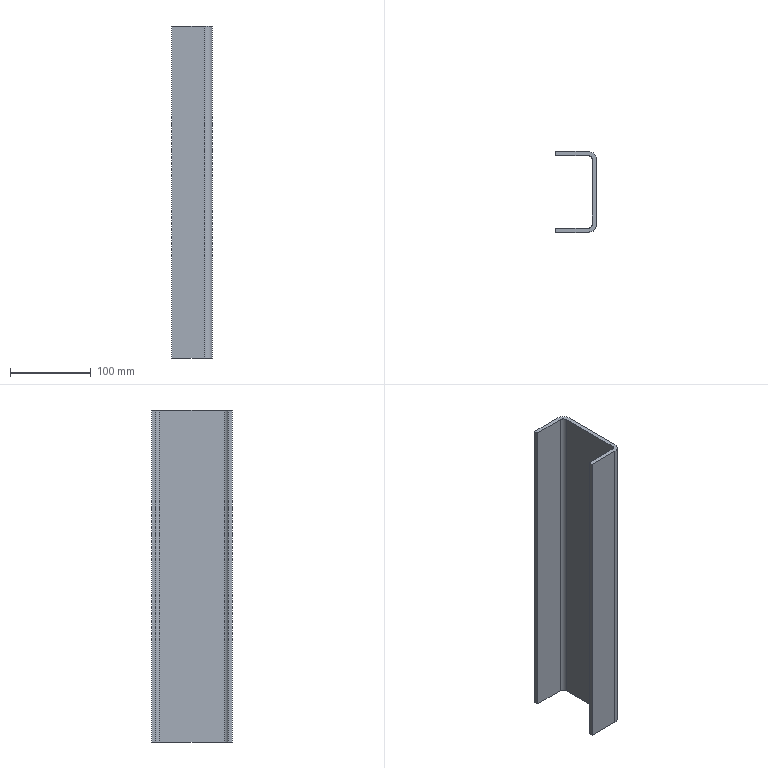Part | STEP file | 1 solid | 14 faces | box 50 x 100 x 410 mm | volume 376302 mm3 | plane 10 | cylinder 4 | commonest cylinder face diameters 10 x2 20 x2
STEP:
#1=CARTESIAN_POINT('',(0.,0.,0.));
#2=DIRECTION('',(0.,0.,1.));
#3=DIRECTION('',(1.,0.,0.));
#4=AXIS2_PLACEMENT_3D('',#1,#2,#3);
#5=CARTESIAN_POINT('',(0.,45.,-205.));
#6=VERTEX_POINT('',#5);
#7=CARTESIAN_POINT('',(0.,45.,205.));
#8=VERTEX_POINT('',#7);
#9=CARTESIAN_POINT('',(0.,45.,205.));
#10=DIRECTION('',(0.,0.,1.));
#11=VECTOR('',#10,1.);
#12=LINE('',#9,#11);
#13=CARTESIAN_POINT('',(0.,45.,205.));
#14=DIRECTION('',(1.,0.,0.));
#15=DIRECTION('',(0.,1.,0.));
#16=AXIS2_PLACEMENT_3D('',#13,#14,#15);
#17=PLANE('',#16);
#18=CARTESIAN_POINT('',(0.,0.));
#19=DIRECTION('',(0.,1.));
#20=VECTOR('',#19,1.);
#21=LINE('',#18,#20);
#22=(GEOMETRIC_REPRESENTATION_CONTEXT(2)PARAMETRIC_REPRESENTATION_CONTEXT()REPRESENTATION_CONTEXT('',''));
#23=DEFINITIONAL_REPRESENTATION('',(#21),#22);
#24=PCURVE('',#17,#23);
#25=CARTESIAN_POINT('',(40.,45.,205.));
#26=DIRECTION('',(0.,1.,0.));
#27=DIRECTION('',(1.,0.,0.));
#28=AXIS2_PLACEMENT_3D('',#25,#26,#27);
#29=PLANE('',#28);
#30=CARTESIAN_POINT('',(-40.,0.));
#31=DIRECTION('',(0.,-1.));
#32=VECTOR('',#31,1.);
#33=LINE('',#30,#32);
#34=(GEOMETRIC_REPRESENTATION_CONTEXT(2)PARAMETRIC_REPRESENTATION_CONTEXT()REPRESENTATION_CONTEXT('',''));
#35=DEFINITIONAL_REPRESENTATION('',(#33),#34);
#36=PCURVE('',#29,#35);
#37=SURFACE_CURVE('',#12,(#24,#36),.PCURVE_S1.);
#38=EDGE_CURVE('',#6,#8,#37,.T.);
#39=ORIENTED_EDGE('',*,*,#38,.T.);
#40=CARTESIAN_POINT('',(0.,50.,205.));
#41=VERTEX_POINT('',#40);
#42=CARTESIAN_POINT('',(0.,40.,205.));
#43=DIRECTION('',(0.,1.,0.));
#44=VECTOR('',#43,1.);
#45=LINE('',#42,#44);
#46=CARTESIAN_POINT('',(-5.,0.));
#47=DIRECTION('',(1.,0.));
#48=VECTOR('',#47,1.);
#49=LINE('',#46,#48);
#50=(GEOMETRIC_REPRESENTATION_CONTEXT(2)PARAMETRIC_REPRESENTATION_CONTEXT()REPRESENTATION_CONTEXT('',''));
#51=DEFINITIONAL_REPRESENTATION('',(#49),#50);
#52=PCURVE('',#17,#51);
#53=CARTESIAN_POINT('',(40.,40.,205.));
#54=DIRECTION('',(0.,0.,-1.));
#55=DIRECTION('',(0.,-1.,0.));
#56=AXIS2_PLACEMENT_3D('',#53,#54,#55);
#57=PLANE('',#56);
#58=CARTESIAN_POINT('',(0.,40.));
#59=DIRECTION('',(-1.,0.));
#60=VECTOR('',#59,1.);
#61=LINE('',#58,#60);
#62=(GEOMETRIC_REPRESENTATION_CONTEXT(2)PARAMETRIC_REPRESENTATION_CONTEXT()REPRESENTATION_CONTEXT('',''));
#63=DEFINITIONAL_REPRESENTATION('',(#61),#62);
#64=PCURVE('',#57,#63);
#65=SURFACE_CURVE('',#45,(#52,#64),.PCURVE_S1.);
#66=EDGE_CURVE('',#8,#41,#65,.T.);
#67=ORIENTED_EDGE('',*,*,#66,.T.);
#68=CARTESIAN_POINT('',(0.,50.,-205.));
#69=VERTEX_POINT('',#68);
#70=CARTESIAN_POINT('',(0.,50.,205.));
#71=DIRECTION('',(0.,0.,-1.));
#72=VECTOR('',#71,1.);
#73=LINE('',#70,#72);
#74=CARTESIAN_POINT('',(5.,0.));
#75=DIRECTION('',(0.,-1.));
#76=VECTOR('',#75,1.);
#77=LINE('',#74,#76);
#78=(GEOMETRIC_REPRESENTATION_CONTEXT(2)PARAMETRIC_REPRESENTATION_CONTEXT()REPRESENTATION_CONTEXT('',''));
#79=DEFINITIONAL_REPRESENTATION('',(#77),#78);
#80=PCURVE('',#17,#79);
#81=CARTESIAN_POINT('',(0.,50.,205.));
#82=DIRECTION('',(0.,-1.,0.));
#83=DIRECTION('',(0.,0.,-1.));
#84=AXIS2_PLACEMENT_3D('',#81,#82,#83);
#85=PLANE('',#84);
#86=CARTESIAN_POINT('',(0.,0.));
#87=DIRECTION('',(1.,0.));
#88=VECTOR('',#87,1.);
#89=LINE('',#86,#88);
#90=(GEOMETRIC_REPRESENTATION_CONTEXT(2)PARAMETRIC_REPRESENTATION_CONTEXT()REPRESENTATION_CONTEXT('',''));
#91=DEFINITIONAL_REPRESENTATION('',(#89),#90);
#92=PCURVE('',#85,#91);
#93=SURFACE_CURVE('',#73,(#80,#92),.PCURVE_S1.);
#94=EDGE_CURVE('',#41,#69,#93,.T.);
#95=ORIENTED_EDGE('',*,*,#94,.T.);
#96=CARTESIAN_POINT('',(0.,40.,-205.));
#97=DIRECTION('',(0.,1.,0.));
#98=VECTOR('',#97,1.);
#99=LINE('',#96,#98);
#100=CARTESIAN_POINT('',(-5.,-410.));
#101=DIRECTION('',(1.,0.));
#102=VECTOR('',#101,1.);
#103=LINE('',#100,#102);
#104=(GEOMETRIC_REPRESENTATION_CONTEXT(2)PARAMETRIC_REPRESENTATION_CONTEXT()REPRESENTATION_CONTEXT('',''));
#105=DEFINITIONAL_REPRESENTATION('',(#103),#104);
#106=PCURVE('',#17,#105);
#107=CARTESIAN_POINT('',(40.,40.,-205.));
#108=DIRECTION('',(0.,0.,-1.));
#109=DIRECTION('',(0.,-1.,0.));
#110=AXIS2_PLACEMENT_3D('',#107,#108,#109);
#111=PLANE('',#110);
#112=CARTESIAN_POINT('',(0.,40.));
#113=DIRECTION('',(-1.,0.));
#114=VECTOR('',#113,1.);
#115=LINE('',#112,#114);
#116=(GEOMETRIC_REPRESENTATION_CONTEXT(2)PARAMETRIC_REPRESENTATION_CONTEXT()REPRESENTATION_CONTEXT('',''));
#117=DEFINITIONAL_REPRESENTATION('',(#115),#116);
#118=PCURVE('',#111,#117);
#119=SURFACE_CURVE('',#99,(#106,#118),.PCURVE_S1.);
#120=EDGE_CURVE('',#6,#69,#119,.T.);
#121=ORIENTED_EDGE('',*,*,#120,.F.);
#122=EDGE_LOOP('',(#39,#67,#95,#121));
#123=FACE_BOUND('',#122,.T.);
#124=ADVANCED_FACE('',(#123),#17,.F.);
#125=ORIENTED_EDGE('',*,*,#94,.F.);
#126=CARTESIAN_POINT('',(40.,50.,205.));
#127=VERTEX_POINT('',#126);
#128=CARTESIAN_POINT('',(40.,50.,205.));
#129=DIRECTION('',(1.,0.,0.));
#130=VECTOR('',#129,1.);
#131=LINE('',#128,#130);
#132=CARTESIAN_POINT('',(0.,40.));
#133=DIRECTION('',(0.,1.));
#134=VECTOR('',#133,1.);
#135=LINE('',#132,#134);
#136=(GEOMETRIC_REPRESENTATION_CONTEXT(2)PARAMETRIC_REPRESENTATION_CONTEXT()REPRESENTATION_CONTEXT('',''));
#137=DEFINITIONAL_REPRESENTATION('',(#135),#136);
#138=PCURVE('',#85,#137);
#139=CARTESIAN_POINT('',(-10.,0.));
#140=DIRECTION('',(0.,-1.));
#141=VECTOR('',#140,1.);
#142=LINE('',#139,#141);
#143=(GEOMETRIC_REPRESENTATION_CONTEXT(2)PARAMETRIC_REPRESENTATION_CONTEXT()REPRESENTATION_CONTEXT('',''));
#144=DEFINITIONAL_REPRESENTATION('',(#142),#143);
#145=PCURVE('',#57,#144);
#146=SURFACE_CURVE('',#131,(#138,#145),.PCURVE_S1.);
#147=EDGE_CURVE('',#41,#127,#146,.T.);
#148=ORIENTED_EDGE('',*,*,#147,.T.);
#149=CARTESIAN_POINT('',(40.,50.,-205.));
#150=VERTEX_POINT('',#149);
#151=CARTESIAN_POINT('',(40.,50.,205.));
#152=DIRECTION('',(0.,0.,1.));
#153=VECTOR('',#152,1.);
#154=LINE('',#151,#153);
#155=CARTESIAN_POINT('',(0.,40.));
#156=DIRECTION('',(-1.,0.));
#157=VECTOR('',#156,1.);
#158=LINE('',#155,#157);
#159=(GEOMETRIC_REPRESENTATION_CONTEXT(2)PARAMETRIC_REPRESENTATION_CONTEXT()REPRESENTATION_CONTEXT('',''));
#160=DEFINITIONAL_REPRESENTATION('',(#158),#159);
#161=PCURVE('',#85,#160);
#162=CARTESIAN_POINT('',(40.,40.,205.));
#163=DIRECTION('',(0.,0.,-1.));
#164=DIRECTION('',(-1.,0.,0.));
#165=AXIS2_PLACEMENT_3D('',#162,#163,#164);
#166=CYLINDRICAL_SURFACE('',#165,10.);
#167=CARTESIAN_POINT('',(1.571,0.));
#168=DIRECTION('',(0.,-1.));
#169=VECTOR('',#168,1.);
#170=LINE('',#167,#169);
#171=(GEOMETRIC_REPRESENTATION_CONTEXT(2)PARAMETRIC_REPRESENTATION_CONTEXT()REPRESENTATION_CONTEXT('',''));
#172=DEFINITIONAL_REPRESENTATION('',(#170),#171);
#173=PCURVE('',#166,#172);
#174=SURFACE_CURVE('',#154,(#161,#173),.PCURVE_S1.);
#175=EDGE_CURVE('',#150,#127,#174,.T.);
#176=ORIENTED_EDGE('',*,*,#175,.F.);
#177=CARTESIAN_POINT('',(40.,50.,-205.));
#178=DIRECTION('',(1.,0.,0.));
#179=VECTOR('',#178,1.);
#180=LINE('',#177,#179);
#181=CARTESIAN_POINT('',(410.,40.));
#182=DIRECTION('',(0.,1.));
#183=VECTOR('',#182,1.);
#184=LINE('',#181,#183);
#185=(GEOMETRIC_REPRESENTATION_CONTEXT(2)PARAMETRIC_REPRESENTATION_CONTEXT()REPRESENTATION_CONTEXT('',''));
#186=DEFINITIONAL_REPRESENTATION('',(#184),#185);
#187=PCURVE('',#85,#186);
#188=CARTESIAN_POINT('',(-10.,0.));
#189=DIRECTION('',(0.,-1.));
#190=VECTOR('',#189,1.);
#191=LINE('',#188,#190);
#192=(GEOMETRIC_REPRESENTATION_CONTEXT(2)PARAMETRIC_REPRESENTATION_CONTEXT()REPRESENTATION_CONTEXT('',''));
#193=DEFINITIONAL_REPRESENTATION('',(#191),#192);
#194=PCURVE('',#111,#193);
#195=SURFACE_CURVE('',#180,(#187,#194),.PCURVE_S1.);
#196=EDGE_CURVE('',#69,#150,#195,.T.);
#197=ORIENTED_EDGE('',*,*,#196,.F.);
#198=EDGE_LOOP('',(#125,#148,#176,#197));
#199=FACE_BOUND('',#198,.T.);
#200=ADVANCED_FACE('',(#199),#85,.F.);
#201=CARTESIAN_POINT('',(50.,40.,205.));
#202=VERTEX_POINT('',#201);
#203=CARTESIAN_POINT('',(40.,40.,205.));
#204=DIRECTION('',(0.,0.,-1.));
#205=DIRECTION('',(-1.,0.,0.));
#206=AXIS2_PLACEMENT_3D('',#203,#204,#205);
#207=CIRCLE('',#206,10.);
#208=CARTESIAN_POINT('',(0.,0.));
#209=DIRECTION('',(1.,0.));
#210=VECTOR('',#209,1.);
#211=LINE('',#208,#210);
#212=(GEOMETRIC_REPRESENTATION_CONTEXT(2)PARAMETRIC_REPRESENTATION_CONTEXT()REPRESENTATION_CONTEXT('',''));
#213=DEFINITIONAL_REPRESENTATION('',(#211),#212);
#214=PCURVE('',#166,#213);
#215=CARTESIAN_POINT('',(0.,0.));
#216=DIRECTION('',(0.,1.));
#217=AXIS2_PLACEMENT_2D('',#215,#216);
#218=CIRCLE('',#217,10.);
#219=(GEOMETRIC_REPRESENTATION_CONTEXT(2)PARAMETRIC_REPRESENTATION_CONTEXT()REPRESENTATION_CONTEXT('',''));
#220=DEFINITIONAL_REPRESENTATION('',(#218),#219);
#221=PCURVE('',#57,#220);
#222=SURFACE_CURVE('',#207,(#214,#221),.PCURVE_S1.);
#223=EDGE_CURVE('',#127,#202,#222,.T.);
#224=ORIENTED_EDGE('',*,*,#223,.T.);
#225=CARTESIAN_POINT('',(50.,40.,-205.));
#226=VERTEX_POINT('',#225);
#227=CARTESIAN_POINT('',(50.,40.,205.));
#228=DIRECTION('',(0.,0.,-1.));
#229=VECTOR('',#228,1.);
#230=LINE('',#227,#229);
#231=CARTESIAN_POINT('',(3.142,0.));
#232=DIRECTION('',(0.,1.));
#233=VECTOR('',#232,1.);
#234=LINE('',#231,#233);
#235=(GEOMETRIC_REPRESENTATION_CONTEXT(2)PARAMETRIC_REPRESENTATION_CONTEXT()REPRESENTATION_CONTEXT('',''));
#236=DEFINITIONAL_REPRESENTATION('',(#234),#235);
#237=PCURVE('',#166,#236);
#238=CARTESIAN_POINT('',(50.,40.,205.));
#239=DIRECTION('',(-1.,0.,0.));
#240=DIRECTION('',(0.,1.,0.));
#241=AXIS2_PLACEMENT_3D('',#238,#239,#240);
#242=PLANE('',#241);
#243=CARTESIAN_POINT('',(0.,0.));
#244=DIRECTION('',(0.,1.));
#245=VECTOR('',#244,1.);
#246=LINE('',#243,#245);
#247=(GEOMETRIC_REPRESENTATION_CONTEXT(2)PARAMETRIC_REPRESENTATION_CONTEXT()REPRESENTATION_CONTEXT('',''));
#248=DEFINITIONAL_REPRESENTATION('',(#246),#247);
#249=PCURVE('',#242,#248);
#250=SURFACE_CURVE('',#230,(#237,#249),.PCURVE_S1.);
#251=EDGE_CURVE('',#202,#226,#250,.T.);
#252=ORIENTED_EDGE('',*,*,#251,.T.);
#253=CARTESIAN_POINT('',(40.,40.,-205.));
#254=DIRECTION('',(0.,0.,-1.));
#255=DIRECTION('',(-1.,0.,0.));
#256=AXIS2_PLACEMENT_3D('',#253,#254,#255);
#257=CIRCLE('',#256,10.);
#258=CARTESIAN_POINT('',(0.,410.));
#259=DIRECTION('',(1.,0.));
#260=VECTOR('',#259,1.);
#261=LINE('',#258,#260);
#262=(GEOMETRIC_REPRESENTATION_CONTEXT(2)PARAMETRIC_REPRESENTATION_CONTEXT()REPRESENTATION_CONTEXT('',''));
#263=DEFINITIONAL_REPRESENTATION('',(#261),#262);
#264=PCURVE('',#166,#263);
#265=CARTESIAN_POINT('',(0.,0.));
#266=DIRECTION('',(0.,1.));
#267=AXIS2_PLACEMENT_2D('',#265,#266);
#268=CIRCLE('',#267,10.);
#269=(GEOMETRIC_REPRESENTATION_CONTEXT(2)PARAMETRIC_REPRESENTATION_CONTEXT()REPRESENTATION_CONTEXT('',''));
#270=DEFINITIONAL_REPRESENTATION('',(#268),#269);
#271=PCURVE('',#111,#270);
#272=SURFACE_CURVE('',#257,(#264,#271),.PCURVE_S1.);
#273=EDGE_CURVE('',#150,#226,#272,.T.);
#274=ORIENTED_EDGE('',*,*,#273,.F.);
#275=ORIENTED_EDGE('',*,*,#175,.T.);
#276=EDGE_LOOP('',(#224,#252,#274,#275));
#277=FACE_BOUND('',#276,.T.);
#278=ADVANCED_FACE('',(#277),#166,.T.);
#279=ORIENTED_EDGE('',*,*,#251,.F.);
#280=CARTESIAN_POINT('',(50.,-40.,205.));
#281=VERTEX_POINT('',#280);
#282=CARTESIAN_POINT('',(50.,40.,205.));
#283=DIRECTION('',(0.,-1.,0.));
#284=VECTOR('',#283,1.);
#285=LINE('',#282,#284);
#286=CARTESIAN_POINT('',(0.,0.));
#287=DIRECTION('',(-1.,0.));
#288=VECTOR('',#287,1.);
#289=LINE('',#286,#288);
#290=(GEOMETRIC_REPRESENTATION_CONTEXT(2)PARAMETRIC_REPRESENTATION_CONTEXT()REPRESENTATION_CONTEXT('',''));
#291=DEFINITIONAL_REPRESENTATION('',(#289),#290);
#292=PCURVE('',#242,#291);
#293=CARTESIAN_POINT('',(0.,-10.));
#294=DIRECTION('',(1.,0.));
#295=VECTOR('',#294,1.);
#296=LINE('',#293,#295);
#297=(GEOMETRIC_REPRESENTATION_CONTEXT(2)PARAMETRIC_REPRESENTATION_CONTEXT()REPRESENTATION_CONTEXT('',''));
#298=DEFINITIONAL_REPRESENTATION('',(#296),#297);
#299=PCURVE('',#57,#298);
#300=SURFACE_CURVE('',#285,(#292,#299),.PCURVE_S1.);
#301=EDGE_CURVE('',#202,#281,#300,.T.);
#302=ORIENTED_EDGE('',*,*,#301,.T.);
#303=CARTESIAN_POINT('',(50.,-40.,-205.));
#304=VERTEX_POINT('',#303);
#305=CARTESIAN_POINT('',(50.,-40.,205.));
#306=DIRECTION('',(0.,0.,1.));
#307=VECTOR('',#306,1.);
#308=LINE('',#305,#307);
#309=CARTESIAN_POINT('',(-80.,0.));
#310=DIRECTION('',(0.,-1.));
#311=VECTOR('',#310,1.);
#312=LINE('',#309,#311);
#313=(GEOMETRIC_REPRESENTATION_CONTEXT(2)PARAMETRIC_REPRESENTATION_CONTEXT()REPRESENTATION_CONTEXT('',''));
#314=DEFINITIONAL_REPRESENTATION('',(#312),#313);
#315=PCURVE('',#242,#314);
#316=CARTESIAN_POINT('',(40.,-40.,205.));
#317=DIRECTION('',(0.,0.,-1.));
#318=DIRECTION('',(-1.,0.,0.));
#319=AXIS2_PLACEMENT_3D('',#316,#317,#318);
#320=CYLINDRICAL_SURFACE('',#319,10.);
#321=CARTESIAN_POINT('',(3.142,0.));
#322=DIRECTION('',(0.,-1.));
#323=VECTOR('',#322,1.);
#324=LINE('',#321,#323);
#325=(GEOMETRIC_REPRESENTATION_CONTEXT(2)PARAMETRIC_REPRESENTATION_CONTEXT()REPRESENTATION_CONTEXT('',''));
#326=DEFINITIONAL_REPRESENTATION('',(#324),#325);
#327=PCURVE('',#320,#326);
#328=SURFACE_CURVE('',#308,(#315,#327),.PCURVE_S1.);
#329=EDGE_CURVE('',#304,#281,#328,.T.);
#330=ORIENTED_EDGE('',*,*,#329,.F.);
#331=CARTESIAN_POINT('',(50.,40.,-205.));
#332=DIRECTION('',(0.,-1.,0.));
#333=VECTOR('',#332,1.);
#334=LINE('',#331,#333);
#335=CARTESIAN_POINT('',(0.,410.));
#336=DIRECTION('',(-1.,0.));
#337=VECTOR('',#336,1.);
#338=LINE('',#335,#337);
#339=(GEOMETRIC_REPRESENTATION_CONTEXT(2)PARAMETRIC_REPRESENTATION_CONTEXT()REPRESENTATION_CONTEXT('',''));
#340=DEFINITIONAL_REPRESENTATION('',(#338),#339);
#341=PCURVE('',#242,#340);
#342=CARTESIAN_POINT('',(0.,-10.));
#343=DIRECTION('',(1.,0.));
#344=VECTOR('',#343,1.);
#345=LINE('',#342,#344);
#346=(GEOMETRIC_REPRESENTATION_CONTEXT(2)PARAMETRIC_REPRESENTATION_CONTEXT()REPRESENTATION_CONTEXT('',''));
#347=DEFINITIONAL_REPRESENTATION('',(#345),#346);
#348=PCURVE('',#111,#347);
#349=SURFACE_CURVE('',#334,(#341,#348),.PCURVE_S1.);
#350=EDGE_CURVE('',#226,#304,#349,.T.);
#351=ORIENTED_EDGE('',*,*,#350,.F.);
#352=EDGE_LOOP('',(#279,#302,#330,#351));
#353=FACE_BOUND('',#352,.T.);
#354=ADVANCED_FACE('',(#353),#242,.F.);
#355=CARTESIAN_POINT('',(40.,-50.,205.));
#356=VERTEX_POINT('',#355);
#357=CARTESIAN_POINT('',(40.,-40.,205.));
#358=DIRECTION('',(0.,0.,-1.));
#359=DIRECTION('',(-1.,0.,0.));
#360=AXIS2_PLACEMENT_3D('',#357,#358,#359);
#361=CIRCLE('',#360,10.);
#362=CARTESIAN_POINT('',(0.,0.));
#363=DIRECTION('',(1.,0.));
#364=VECTOR('',#363,1.);
#365=LINE('',#362,#364);
#366=(GEOMETRIC_REPRESENTATION_CONTEXT(2)PARAMETRIC_REPRESENTATION_CONTEXT()REPRESENTATION_CONTEXT('',''));
#367=DEFINITIONAL_REPRESENTATION('',(#365),#366);
#368=PCURVE('',#320,#367);
#369=CARTESIAN_POINT('',(80.,0.));
#370=DIRECTION('',(0.,1.));
#371=AXIS2_PLACEMENT_2D('',#369,#370);
#372=CIRCLE('',#371,10.);
#373=(GEOMETRIC_REPRESENTATION_CONTEXT(2)PARAMETRIC_REPRESENTATION_CONTEXT()REPRESENTATION_CONTEXT('',''));
#374=DEFINITIONAL_REPRESENTATION('',(#372),#373);
#375=PCURVE('',#57,#374);
#376=SURFACE_CURVE('',#361,(#368,#375),.PCURVE_S1.);
#377=EDGE_CURVE('',#281,#356,#376,.T.);
#378=ORIENTED_EDGE('',*,*,#377,.T.);
#379=CARTESIAN_POINT('',(40.,-50.,-205.));
#380=VERTEX_POINT('',#379);
#381=CARTESIAN_POINT('',(40.,-50.,205.));
#382=DIRECTION('',(0.,0.,-1.));
#383=VECTOR('',#382,1.);
#384=LINE('',#381,#383);
#385=CARTESIAN_POINT('',(4.712,0.));
#386=DIRECTION('',(0.,1.));
#387=VECTOR('',#386,1.);
#388=LINE('',#385,#387);
#389=(GEOMETRIC_REPRESENTATION_CONTEXT(2)PARAMETRIC_REPRESENTATION_CONTEXT()REPRESENTATION_CONTEXT('',''));
#390=DEFINITIONAL_REPRESENTATION('',(#388),#389);
#391=PCURVE('',#320,#390);
#392=CARTESIAN_POINT('',(40.,-50.,205.));
#393=DIRECTION('',(0.,1.,0.));
#394=DIRECTION('',(1.,0.,0.));
#395=AXIS2_PLACEMENT_3D('',#392,#393,#394);
#396=PLANE('',#395);
#397=CARTESIAN_POINT('',(0.,0.));
#398=DIRECTION('',(0.,1.));
#399=VECTOR('',#398,1.);
#400=LINE('',#397,#399);
#401=(GEOMETRIC_REPRESENTATION_CONTEXT(2)PARAMETRIC_REPRESENTATION_CONTEXT()REPRESENTATION_CONTEXT('',''));
#402=DEFINITIONAL_REPRESENTATION('',(#400),#401);
#403=PCURVE('',#396,#402);
#404=SURFACE_CURVE('',#384,(#391,#403),.PCURVE_S1.);
#405=EDGE_CURVE('',#356,#380,#404,.T.);
#406=ORIENTED_EDGE('',*,*,#405,.T.);
#407=CARTESIAN_POINT('',(40.,-40.,-205.));
#408=DIRECTION('',(0.,0.,-1.));
#409=DIRECTION('',(-1.,0.,0.));
#410=AXIS2_PLACEMENT_3D('',#407,#408,#409);
#411=CIRCLE('',#410,10.);
#412=CARTESIAN_POINT('',(0.,410.));
#413=DIRECTION('',(1.,0.));
#414=VECTOR('',#413,1.);
#415=LINE('',#412,#414);
#416=(GEOMETRIC_REPRESENTATION_CONTEXT(2)PARAMETRIC_REPRESENTATION_CONTEXT()REPRESENTATION_CONTEXT('',''));
#417=DEFINITIONAL_REPRESENTATION('',(#415),#416);
#418=PCURVE('',#320,#417);
#419=CARTESIAN_POINT('',(80.,0.));
#420=DIRECTION('',(0.,1.));
#421=AXIS2_PLACEMENT_2D('',#419,#420);
#422=CIRCLE('',#421,10.);
#423=(GEOMETRIC_REPRESENTATION_CONTEXT(2)PARAMETRIC_REPRESENTATION_CONTEXT()REPRESENTATION_CONTEXT('',''));
#424=DEFINITIONAL_REPRESENTATION('',(#422),#423);
#425=PCURVE('',#111,#424);
#426=SURFACE_CURVE('',#411,(#418,#425),.PCURVE_S1.);
#427=EDGE_CURVE('',#304,#380,#426,.T.);
#428=ORIENTED_EDGE('',*,*,#427,.F.);
#429=ORIENTED_EDGE('',*,*,#329,.T.);
#430=EDGE_LOOP('',(#378,#406,#428,#429));
#431=FACE_BOUND('',#430,.T.);
#432=ADVANCED_FACE('',(#431),#320,.T.);
#433=ORIENTED_EDGE('',*,*,#405,.F.);
#434=CARTESIAN_POINT('',(0.,-50.,205.));
#435=VERTEX_POINT('',#434);
#436=CARTESIAN_POINT('',(40.,-50.,205.));
#437=DIRECTION('',(-1.,0.,0.));
#438=VECTOR('',#437,1.);
#439=LINE('',#436,#438);
#440=CARTESIAN_POINT('',(0.,0.));
#441=DIRECTION('',(-1.,0.));
#442=VECTOR('',#441,1.);
#443=LINE('',#440,#442);
#444=(GEOMETRIC_REPRESENTATION_CONTEXT(2)PARAMETRIC_REPRESENTATION_CONTEXT()REPRESENTATION_CONTEXT('',''));
#445=DEFINITIONAL_REPRESENTATION('',(#443),#444);
#446=PCURVE('',#396,#445);
#447=CARTESIAN_POINT('',(90.,0.));
#448=DIRECTION('',(0.,1.));
#449=VECTOR('',#448,1.);
#450=LINE('',#447,#449);
#451=(GEOMETRIC_REPRESENTATION_CONTEXT(2)PARAMETRIC_REPRESENTATION_CONTEXT()REPRESENTATION_CONTEXT('',''));
#452=DEFINITIONAL_REPRESENTATION('',(#450),#451);
#453=PCURVE('',#57,#452);
#454=SURFACE_CURVE('',#439,(#446,#453),.PCURVE_S1.);
#455=EDGE_CURVE('',#356,#435,#454,.T.);
#456=ORIENTED_EDGE('',*,*,#455,.T.);
#457=CARTESIAN_POINT('',(0.,-50.,-205.));
#458=VERTEX_POINT('',#457);
#459=CARTESIAN_POINT('',(0.,-50.,205.));
#460=DIRECTION('',(0.,0.,-1.));
#461=VECTOR('',#460,1.);
#462=LINE('',#459,#461);
#463=CARTESIAN_POINT('',(-40.,0.));
#464=DIRECTION('',(0.,1.));
#465=VECTOR('',#464,1.);
#466=LINE('',#463,#465);
#467=(GEOMETRIC_REPRESENTATION_CONTEXT(2)PARAMETRIC_REPRESENTATION_CONTEXT()REPRESENTATION_CONTEXT('',''));
#468=DEFINITIONAL_REPRESENTATION('',(#466),#467);
#469=PCURVE('',#396,#468);
#470=CARTESIAN_POINT('',(0.,-50.,205.));
#471=DIRECTION('',(1.,0.,0.));
#472=DIRECTION('',(0.,1.,0.));
#473=AXIS2_PLACEMENT_3D('',#470,#471,#472);
#474=PLANE('',#473);
#475=CARTESIAN_POINT('',(0.,0.));
#476=DIRECTION('',(0.,-1.));
#477=VECTOR('',#476,1.);
#478=LINE('',#475,#477);
#479=(GEOMETRIC_REPRESENTATION_CONTEXT(2)PARAMETRIC_REPRESENTATION_CONTEXT()REPRESENTATION_CONTEXT('',''));
#480=DEFINITIONAL_REPRESENTATION('',(#478),#479);
#481=PCURVE('',#474,#480);
#482=SURFACE_CURVE('',#462,(#469,#481),.PCURVE_S1.);
#483=EDGE_CURVE('',#435,#458,#482,.T.);
#484=ORIENTED_EDGE('',*,*,#483,.T.);
#485=CARTESIAN_POINT('',(40.,-50.,-205.));
#486=DIRECTION('',(-1.,0.,0.));
#487=VECTOR('',#486,1.);
#488=LINE('',#485,#487);
#489=CARTESIAN_POINT('',(0.,410.));
#490=DIRECTION('',(-1.,0.));
#491=VECTOR('',#490,1.);
#492=LINE('',#489,#491);
#493=(GEOMETRIC_REPRESENTATION_CONTEXT(2)PARAMETRIC_REPRESENTATION_CONTEXT()REPRESENTATION_CONTEXT('',''));
#494=DEFINITIONAL_REPRESENTATION('',(#492),#493);
#495=PCURVE('',#396,#494);
#496=CARTESIAN_POINT('',(90.,0.));
#497=DIRECTION('',(0.,1.));
#498=VECTOR('',#497,1.);
#499=LINE('',#496,#498);
#500=(GEOMETRIC_REPRESENTATION_CONTEXT(2)PARAMETRIC_REPRESENTATION_CONTEXT()REPRESENTATION_CONTEXT('',''));
#501=DEFINITIONAL_REPRESENTATION('',(#499),#500);
#502=PCURVE('',#111,#501);
#503=SURFACE_CURVE('',#488,(#495,#502),.PCURVE_S1.);
#504=EDGE_CURVE('',#380,#458,#503,.T.);
#505=ORIENTED_EDGE('',*,*,#504,.F.);
#506=EDGE_LOOP('',(#433,#456,#484,#505));
#507=FACE_BOUND('',#506,.T.);
#508=ADVANCED_FACE('',(#507),#396,.F.);
#509=ORIENTED_EDGE('',*,*,#483,.F.);
#510=CARTESIAN_POINT('',(0.,-45.,205.));
#511=VERTEX_POINT('',#510);
#512=CARTESIAN_POINT('',(0.,40.,205.));
#513=DIRECTION('',(0.,1.,0.));
#514=VECTOR('',#513,1.);
#515=LINE('',#512,#514);
#516=CARTESIAN_POINT('',(90.,0.));
#517=DIRECTION('',(1.,0.));
#518=VECTOR('',#517,1.);
#519=LINE('',#516,#518);
#520=(GEOMETRIC_REPRESENTATION_CONTEXT(2)PARAMETRIC_REPRESENTATION_CONTEXT()REPRESENTATION_CONTEXT('',''));
#521=DEFINITIONAL_REPRESENTATION('',(#519),#520);
#522=PCURVE('',#474,#521);
#523=CARTESIAN_POINT('',(0.,40.));
#524=DIRECTION('',(-1.,0.));
#525=VECTOR('',#524,1.);
#526=LINE('',#523,#525);
#527=(GEOMETRIC_REPRESENTATION_CONTEXT(2)PARAMETRIC_REPRESENTATION_CONTEXT()REPRESENTATION_CONTEXT('',''));
#528=DEFINITIONAL_REPRESENTATION('',(#526),#527);
#529=PCURVE('',#57,#528);
#530=SURFACE_CURVE('',#515,(#522,#529),.PCURVE_S1.);
#531=EDGE_CURVE('',#435,#511,#530,.T.);
#532=ORIENTED_EDGE('',*,*,#531,.T.);
#533=CARTESIAN_POINT('',(0.,-45.,-205.));
#534=VERTEX_POINT('',#533);
#535=CARTESIAN_POINT('',(0.,-45.,205.));
#536=DIRECTION('',(0.,0.,-1.));
#537=VECTOR('',#536,1.);
#538=LINE('',#535,#537);
#539=CARTESIAN_POINT('',(5.,0.));
#540=DIRECTION('',(0.,-1.));
#541=VECTOR('',#540,1.);
#542=LINE('',#539,#541);
#543=(GEOMETRIC_REPRESENTATION_CONTEXT(2)PARAMETRIC_REPRESENTATION_CONTEXT()REPRESENTATION_CONTEXT('',''));
#544=DEFINITIONAL_REPRESENTATION('',(#542),#543);
#545=PCURVE('',#474,#544);
#546=CARTESIAN_POINT('',(0.,-45.,205.));
#547=DIRECTION('',(0.,-1.,0.));
#548=DIRECTION('',(0.,0.,-1.));
#549=AXIS2_PLACEMENT_3D('',#546,#547,#548);
#550=PLANE('',#549);
#551=CARTESIAN_POINT('',(0.,0.));
#552=DIRECTION('',(1.,0.));
#553=VECTOR('',#552,1.);
#554=LINE('',#551,#553);
#555=(GEOMETRIC_REPRESENTATION_CONTEXT(2)PARAMETRIC_REPRESENTATION_CONTEXT()REPRESENTATION_CONTEXT('',''));
#556=DEFINITIONAL_REPRESENTATION('',(#554),#555);
#557=PCURVE('',#550,#556);
#558=SURFACE_CURVE('',#538,(#545,#557),.PCURVE_S1.);
#559=EDGE_CURVE('',#511,#534,#558,.T.);
#560=ORIENTED_EDGE('',*,*,#559,.T.);
#561=CARTESIAN_POINT('',(0.,40.,-205.));
#562=DIRECTION('',(0.,1.,0.));
#563=VECTOR('',#562,1.);
#564=LINE('',#561,#563);
#565=CARTESIAN_POINT('',(90.,-410.));
#566=DIRECTION('',(1.,0.));
#567=VECTOR('',#566,1.);
#568=LINE('',#565,#567);
#569=(GEOMETRIC_REPRESENTATION_CONTEXT(2)PARAMETRIC_REPRESENTATION_CONTEXT()REPRESENTATION_CONTEXT('',''));
#570=DEFINITIONAL_REPRESENTATION('',(#568),#569);
#571=PCURVE('',#474,#570);
#572=CARTESIAN_POINT('',(0.,40.));
#573=DIRECTION('',(-1.,0.));
#574=VECTOR('',#573,1.);
#575=LINE('',#572,#574);
#576=(GEOMETRIC_REPRESENTATION_CONTEXT(2)PARAMETRIC_REPRESENTATION_CONTEXT()REPRESENTATION_CONTEXT('',''));
#577=DEFINITIONAL_REPRESENTATION('',(#575),#576);
#578=PCURVE('',#111,#577);
#579=SURFACE_CURVE('',#564,(#571,#578),.PCURVE_S1.);
#580=EDGE_CURVE('',#458,#534,#579,.T.);
#581=ORIENTED_EDGE('',*,*,#580,.F.);
#582=EDGE_LOOP('',(#509,#532,#560,#581));
#583=FACE_BOUND('',#582,.T.);
#584=ADVANCED_FACE('',(#583),#474,.F.);
#585=ORIENTED_EDGE('',*,*,#559,.F.);
#586=CARTESIAN_POINT('',(40.,-45.,205.));
#587=VERTEX_POINT('',#586);
#588=CARTESIAN_POINT('',(40.,-45.,205.));
#589=DIRECTION('',(1.,0.,0.));
#590=VECTOR('',#589,1.);
#591=LINE('',#588,#590);
#592=CARTESIAN_POINT('',(0.,40.));
#593=DIRECTION('',(0.,1.));
#594=VECTOR('',#593,1.);
#595=LINE('',#592,#594);
#596=(GEOMETRIC_REPRESENTATION_CONTEXT(2)PARAMETRIC_REPRESENTATION_CONTEXT()REPRESENTATION_CONTEXT('',''));
#597=DEFINITIONAL_REPRESENTATION('',(#595),#596);
#598=PCURVE('',#550,#597);
#599=CARTESIAN_POINT('',(85.,0.));
#600=DIRECTION('',(0.,-1.));
#601=VECTOR('',#600,1.);
#602=LINE('',#599,#601);
#603=(GEOMETRIC_REPRESENTATION_CONTEXT(2)PARAMETRIC_REPRESENTATION_CONTEXT()REPRESENTATION_CONTEXT('',''));
#604=DEFINITIONAL_REPRESENTATION('',(#602),#603);
#605=PCURVE('',#57,#604);
#606=SURFACE_CURVE('',#591,(#598,#605),.PCURVE_S1.);
#607=EDGE_CURVE('',#511,#587,#606,.T.);
#608=ORIENTED_EDGE('',*,*,#607,.T.);
#609=CARTESIAN_POINT('',(40.,-45.,-205.));
#610=VERTEX_POINT('',#609);
#611=CARTESIAN_POINT('',(40.,-45.,205.));
#612=DIRECTION('',(0.,0.,-1.));
#613=VECTOR('',#612,1.);
#614=LINE('',#611,#613);
#615=CARTESIAN_POINT('',(0.,40.));
#616=DIRECTION('',(1.,0.));
#617=VECTOR('',#616,1.);
#618=LINE('',#615,#617);
#619=(GEOMETRIC_REPRESENTATION_CONTEXT(2)PARAMETRIC_REPRESENTATION_CONTEXT()REPRESENTATION_CONTEXT('',''));
#620=DEFINITIONAL_REPRESENTATION('',(#618),#619);
#621=PCURVE('',#550,#620);
#622=CARTESIAN_POINT('',(40.,-40.,205.));
#623=DIRECTION('',(0.,0.,-1.));
#624=DIRECTION('',(-1.,0.,0.));
#625=AXIS2_PLACEMENT_3D('',#622,#623,#624);
#626=CYLINDRICAL_SURFACE('',#625,5.);
#627=CARTESIAN_POINT('',(4.712,0.));
#628=DIRECTION('',(0.,1.));
#629=VECTOR('',#628,1.);
#630=LINE('',#627,#629);
#631=(GEOMETRIC_REPRESENTATION_CONTEXT(2)PARAMETRIC_REPRESENTATION_CONTEXT()REPRESENTATION_CONTEXT('',''));
#632=DEFINITIONAL_REPRESENTATION('',(#630),#631);
#633=PCURVE('',#626,#632);
#634=SURFACE_CURVE('',#614,(#621,#633),.PCURVE_S1.);
#635=EDGE_CURVE('',#587,#610,#634,.T.);
#636=ORIENTED_EDGE('',*,*,#635,.T.);
#637=CARTESIAN_POINT('',(40.,-45.,-205.));
#638=DIRECTION('',(1.,0.,0.));
#639=VECTOR('',#638,1.);
#640=LINE('',#637,#639);
#641=CARTESIAN_POINT('',(410.,40.));
#642=DIRECTION('',(0.,1.));
#643=VECTOR('',#642,1.);
#644=LINE('',#641,#643);
#645=(GEOMETRIC_REPRESENTATION_CONTEXT(2)PARAMETRIC_REPRESENTATION_CONTEXT()REPRESENTATION_CONTEXT('',''));
#646=DEFINITIONAL_REPRESENTATION('',(#644),#645);
#647=PCURVE('',#550,#646);
#648=CARTESIAN_POINT('',(85.,0.));
#649=DIRECTION('',(0.,-1.));
#650=VECTOR('',#649,1.);
#651=LINE('',#648,#650);
#652=(GEOMETRIC_REPRESENTATION_CONTEXT(2)PARAMETRIC_REPRESENTATION_CONTEXT()REPRESENTATION_CONTEXT('',''));
#653=DEFINITIONAL_REPRESENTATION('',(#651),#652);
#654=PCURVE('',#111,#653);
#655=SURFACE_CURVE('',#640,(#647,#654),.PCURVE_S1.);
#656=EDGE_CURVE('',#534,#610,#655,.T.);
#657=ORIENTED_EDGE('',*,*,#656,.F.);
#658=EDGE_LOOP('',(#585,#608,#636,#657));
#659=FACE_BOUND('',#658,.T.);
#660=ADVANCED_FACE('',(#659),#550,.F.);
#661=CARTESIAN_POINT('',(40.,45.,-205.));
#662=VERTEX_POINT('',#661);
#663=CARTESIAN_POINT('',(40.,45.,205.));
#664=VERTEX_POINT('',#663);
#665=CARTESIAN_POINT('',(40.,45.,205.));
#666=DIRECTION('',(0.,0.,1.));
#667=VECTOR('',#666,1.);
#668=LINE('',#665,#667);
#669=CARTESIAN_POINT('',(0.,0.));
#670=DIRECTION('',(0.,-1.));
#671=VECTOR('',#670,1.);
#672=LINE('',#669,#671);
#673=(GEOMETRIC_REPRESENTATION_CONTEXT(2)PARAMETRIC_REPRESENTATION_CONTEXT()REPRESENTATION_CONTEXT('',''));
#674=DEFINITIONAL_REPRESENTATION('',(#672),#673);
#675=PCURVE('',#29,#674);
#676=CARTESIAN_POINT('',(40.,40.,205.));
#677=DIRECTION('',(0.,0.,-1.));
#678=DIRECTION('',(-1.,0.,0.));
#679=AXIS2_PLACEMENT_3D('',#676,#677,#678);
#680=CYLINDRICAL_SURFACE('',#679,5.);
#681=CARTESIAN_POINT('',(1.571,0.));
#682=DIRECTION('',(0.,-1.));
#683=VECTOR('',#682,1.);
#684=LINE('',#681,#683);
#685=(GEOMETRIC_REPRESENTATION_CONTEXT(2)PARAMETRIC_REPRESENTATION_CONTEXT()REPRESENTATION_CONTEXT('',''));
#686=DEFINITIONAL_REPRESENTATION('',(#684),#685);
#687=PCURVE('',#680,#686);
#688=SURFACE_CURVE('',#668,(#675,#687),.PCURVE_S1.);
#689=EDGE_CURVE('',#662,#664,#688,.T.);
#690=ORIENTED_EDGE('',*,*,#689,.T.);
#691=CARTESIAN_POINT('',(40.,45.,205.));
#692=DIRECTION('',(-1.,0.,0.));
#693=VECTOR('',#692,1.);
#694=LINE('',#691,#693);
#695=CARTESIAN_POINT('',(0.,0.));
#696=DIRECTION('',(-1.,0.));
#697=VECTOR('',#696,1.);
#698=LINE('',#695,#697);
#699=(GEOMETRIC_REPRESENTATION_CONTEXT(2)PARAMETRIC_REPRESENTATION_CONTEXT()REPRESENTATION_CONTEXT('',''));
#700=DEFINITIONAL_REPRESENTATION('',(#698),#699);
#701=PCURVE('',#29,#700);
#702=CARTESIAN_POINT('',(-5.,0.));
#703=DIRECTION('',(0.,1.));
#704=VECTOR('',#703,1.);
#705=LINE('',#702,#704);
#706=(GEOMETRIC_REPRESENTATION_CONTEXT(2)PARAMETRIC_REPRESENTATION_CONTEXT()REPRESENTATION_CONTEXT('',''));
#707=DEFINITIONAL_REPRESENTATION('',(#705),#706);
#708=PCURVE('',#57,#707);
#709=SURFACE_CURVE('',#694,(#701,#708),.PCURVE_S1.);
#710=EDGE_CURVE('',#664,#8,#709,.T.);
#711=ORIENTED_EDGE('',*,*,#710,.T.);
#712=ORIENTED_EDGE('',*,*,#38,.F.);
#713=CARTESIAN_POINT('',(40.,45.,-205.));
#714=DIRECTION('',(-1.,0.,0.));
#715=VECTOR('',#714,1.);
#716=LINE('',#713,#715);
#717=CARTESIAN_POINT('',(0.,410.));
#718=DIRECTION('',(-1.,0.));
#719=VECTOR('',#718,1.);
#720=LINE('',#717,#719);
#721=(GEOMETRIC_REPRESENTATION_CONTEXT(2)PARAMETRIC_REPRESENTATION_CONTEXT()REPRESENTATION_CONTEXT('',''));
#722=DEFINITIONAL_REPRESENTATION('',(#720),#721);
#723=PCURVE('',#29,#722);
#724=CARTESIAN_POINT('',(-5.,0.));
#725=DIRECTION('',(0.,1.));
#726=VECTOR('',#725,1.);
#727=LINE('',#724,#726);
#728=(GEOMETRIC_REPRESENTATION_CONTEXT(2)PARAMETRIC_REPRESENTATION_CONTEXT()REPRESENTATION_CONTEXT('',''));
#729=DEFINITIONAL_REPRESENTATION('',(#727),#728);
#730=PCURVE('',#111,#729);
#731=SURFACE_CURVE('',#716,(#723,#730),.PCURVE_S1.);
#732=EDGE_CURVE('',#662,#6,#731,.T.);
#733=ORIENTED_EDGE('',*,*,#732,.F.);
#734=EDGE_LOOP('',(#690,#711,#712,#733));
#735=FACE_BOUND('',#734,.T.);
#736=ADVANCED_FACE('',(#735),#29,.F.);
#737=CARTESIAN_POINT('',(45.,40.,-205.));
#738=VERTEX_POINT('',#737);
#739=CARTESIAN_POINT('',(40.,40.,-205.));
#740=DIRECTION('',(0.,0.,1.));
#741=DIRECTION('',(-1.,0.,0.));
#742=AXIS2_PLACEMENT_3D('',#739,#740,#741);
#743=CIRCLE('',#742,5.);
#744=CARTESIAN_POINT('',(6.283,410.));
#745=DIRECTION('',(-1.,0.));
#746=VECTOR('',#745,1.);
#747=LINE('',#744,#746);
#748=(GEOMETRIC_REPRESENTATION_CONTEXT(2)PARAMETRIC_REPRESENTATION_CONTEXT()REPRESENTATION_CONTEXT('',''));
#749=DEFINITIONAL_REPRESENTATION('',(#747),#748);
#750=PCURVE('',#680,#749);
#751=CARTESIAN_POINT('',(0.,5.));
#752=CARTESIAN_POINT('',(8.66,5.));
#753=CARTESIAN_POINT('',(4.33,-2.5));
#754=CARTESIAN_POINT('',(0.,-10.));
#755=CARTESIAN_POINT('',(-4.33,-2.5));
#756=CARTESIAN_POINT('',(-8.66,5.));
#757=CARTESIAN_POINT('',(0.,5.));
#758=(BOUNDED_CURVE()B_SPLINE_CURVE(2,(#751,#752,#753,#754,#755,#756,#757),.UNSPECIFIED.,.T.,.F.)B_SPLINE_CURVE_WITH_KNOTS((1,2,2,2,2,1),(-2.094,0.,2.094,4.189,6.283,8.378),.UNSPECIFIED.)CURVE()GEOMETRIC_REPRESENTATION_ITEM()RATIONAL_B_SPLINE_CURVE((1.,0.5,1.,0.5,1.,0.5,1.))REPRESENTATION_ITEM(''));
#759=(GEOMETRIC_REPRESENTATION_CONTEXT(2)PARAMETRIC_REPRESENTATION_CONTEXT()REPRESENTATION_CONTEXT('',''));
#760=DEFINITIONAL_REPRESENTATION('',(#758),#759);
#761=PCURVE('',#111,#760);
#762=SURFACE_CURVE('',#743,(#750,#761),.PCURVE_S1.);
#763=EDGE_CURVE('',#738,#662,#762,.T.);
#764=ORIENTED_EDGE('',*,*,#763,.T.);
#765=ORIENTED_EDGE('',*,*,#689,.T.);
#766=CARTESIAN_POINT('',(45.,40.,205.));
#767=VERTEX_POINT('',#766);
#768=CARTESIAN_POINT('',(40.,40.,205.));
#769=DIRECTION('',(0.,0.,1.));
#770=DIRECTION('',(-1.,0.,0.));
#771=AXIS2_PLACEMENT_3D('',#768,#769,#770);
#772=CIRCLE('',#771,5.);
#773=CARTESIAN_POINT('',(6.283,0.));
#774=DIRECTION('',(-1.,0.));
#775=VECTOR('',#774,1.);
#776=LINE('',#773,#775);
#777=(GEOMETRIC_REPRESENTATION_CONTEXT(2)PARAMETRIC_REPRESENTATION_CONTEXT()REPRESENTATION_CONTEXT('',''));
#778=DEFINITIONAL_REPRESENTATION('',(#776),#777);
#779=PCURVE('',#680,#778);
#780=CARTESIAN_POINT('',(0.,5.));
#781=CARTESIAN_POINT('',(8.66,5.));
#782=CARTESIAN_POINT('',(4.33,-2.5));
#783=CARTESIAN_POINT('',(0.,-10.));
#784=CARTESIAN_POINT('',(-4.33,-2.5));
#785=CARTESIAN_POINT('',(-8.66,5.));
#786=CARTESIAN_POINT('',(0.,5.));
#787=(BOUNDED_CURVE()B_SPLINE_CURVE(2,(#780,#781,#782,#783,#784,#785,#786),.UNSPECIFIED.,.T.,.F.)B_SPLINE_CURVE_WITH_KNOTS((1,2,2,2,2,1),(-2.094,0.,2.094,4.189,6.283,8.378),.UNSPECIFIED.)CURVE()GEOMETRIC_REPRESENTATION_ITEM()RATIONAL_B_SPLINE_CURVE((1.,0.5,1.,0.5,1.,0.5,1.))REPRESENTATION_ITEM(''));
#788=(GEOMETRIC_REPRESENTATION_CONTEXT(2)PARAMETRIC_REPRESENTATION_CONTEXT()REPRESENTATION_CONTEXT('',''));
#789=DEFINITIONAL_REPRESENTATION('',(#787),#788);
#790=PCURVE('',#57,#789);
#791=SURFACE_CURVE('',#772,(#779,#790),.PCURVE_S1.);
#792=EDGE_CURVE('',#767,#664,#791,.T.);
#793=ORIENTED_EDGE('',*,*,#792,.F.);
#794=CARTESIAN_POINT('',(45.,40.,205.));
#795=DIRECTION('',(0.,0.,1.));
#796=VECTOR('',#795,1.);
#797=LINE('',#794,#796);
#798=CARTESIAN_POINT('',(3.142,0.));
#799=DIRECTION('',(0.,-1.));
#800=VECTOR('',#799,1.);
#801=LINE('',#798,#800);
#802=(GEOMETRIC_REPRESENTATION_CONTEXT(2)PARAMETRIC_REPRESENTATION_CONTEXT()REPRESENTATION_CONTEXT('',''));
#803=DEFINITIONAL_REPRESENTATION('',(#801),#802);
#804=PCURVE('',#680,#803);
#805=CARTESIAN_POINT('',(45.,-40.,205.));
#806=DIRECTION('',(1.,0.,0.));
#807=DIRECTION('',(0.,1.,0.));
#808=AXIS2_PLACEMENT_3D('',#805,#806,#807);
#809=PLANE('',#808);
#810=CARTESIAN_POINT('',(80.,0.));
#811=DIRECTION('',(0.,1.));
#812=VECTOR('',#811,1.);
#813=LINE('',#810,#812);
#814=(GEOMETRIC_REPRESENTATION_CONTEXT(2)PARAMETRIC_REPRESENTATION_CONTEXT()REPRESENTATION_CONTEXT('',''));
#815=DEFINITIONAL_REPRESENTATION('',(#813),#814);
#816=PCURVE('',#809,#815);
#817=SURFACE_CURVE('',#797,(#804,#816),.PCURVE_S1.);
#818=EDGE_CURVE('',#738,#767,#817,.T.);
#819=ORIENTED_EDGE('',*,*,#818,.F.);
#820=EDGE_LOOP('',(#764,#765,#793,#819));
#821=FACE_BOUND('',#820,.F.);
#822=ADVANCED_FACE('',(#821),#680,.F.);
#823=ORIENTED_EDGE('',*,*,#710,.F.);
#824=ORIENTED_EDGE('',*,*,#792,.F.);
#825=CARTESIAN_POINT('',(45.,-40.,205.));
#826=VERTEX_POINT('',#825);
#827=CARTESIAN_POINT('',(45.,-40.,205.));
#828=DIRECTION('',(0.,-1.,0.));
#829=VECTOR('',#828,1.);
#830=LINE('',#827,#829);
#831=CARTESIAN_POINT('',(80.,-5.));
#832=DIRECTION('',(1.,0.));
#833=VECTOR('',#832,1.);
#834=LINE('',#831,#833);
#835=(GEOMETRIC_REPRESENTATION_CONTEXT(2)PARAMETRIC_REPRESENTATION_CONTEXT()REPRESENTATION_CONTEXT('',''));
#836=DEFINITIONAL_REPRESENTATION('',(#834),#835);
#837=PCURVE('',#57,#836);
#838=CARTESIAN_POINT('',(0.,0.));
#839=DIRECTION('',(-1.,0.));
#840=VECTOR('',#839,1.);
#841=LINE('',#838,#840);
#842=(GEOMETRIC_REPRESENTATION_CONTEXT(2)PARAMETRIC_REPRESENTATION_CONTEXT()REPRESENTATION_CONTEXT('',''));
#843=DEFINITIONAL_REPRESENTATION('',(#841),#842);
#844=PCURVE('',#809,#843);
#845=SURFACE_CURVE('',#830,(#837,#844),.PCURVE_S1.);
#846=EDGE_CURVE('',#767,#826,#845,.T.);
#847=ORIENTED_EDGE('',*,*,#846,.T.);
#848=CARTESIAN_POINT('',(40.,-40.,205.));
#849=DIRECTION('',(0.,0.,-1.));
#850=DIRECTION('',(-1.,0.,0.));
#851=AXIS2_PLACEMENT_3D('',#848,#849,#850);
#852=CIRCLE('',#851,5.);
#853=CARTESIAN_POINT('',(80.,0.));
#854=DIRECTION('',(0.,1.));
#855=AXIS2_PLACEMENT_2D('',#853,#854);
#856=CIRCLE('',#855,5.);
#857=(GEOMETRIC_REPRESENTATION_CONTEXT(2)PARAMETRIC_REPRESENTATION_CONTEXT()REPRESENTATION_CONTEXT('',''));
#858=DEFINITIONAL_REPRESENTATION('',(#856),#857);
#859=PCURVE('',#57,#858);
#860=CARTESIAN_POINT('',(0.,0.));
#861=DIRECTION('',(1.,0.));
#862=VECTOR('',#861,1.);
#863=LINE('',#860,#862);
#864=(GEOMETRIC_REPRESENTATION_CONTEXT(2)PARAMETRIC_REPRESENTATION_CONTEXT()REPRESENTATION_CONTEXT('',''));
#865=DEFINITIONAL_REPRESENTATION('',(#863),#864);
#866=PCURVE('',#626,#865);
#867=SURFACE_CURVE('',#852,(#859,#866),.PCURVE_S1.);
#868=EDGE_CURVE('',#826,#587,#867,.T.);
#869=ORIENTED_EDGE('',*,*,#868,.T.);
#870=ORIENTED_EDGE('',*,*,#607,.F.);
#871=ORIENTED_EDGE('',*,*,#531,.F.);
#872=ORIENTED_EDGE('',*,*,#455,.F.);
#873=ORIENTED_EDGE('',*,*,#377,.F.);
#874=ORIENTED_EDGE('',*,*,#301,.F.);
#875=ORIENTED_EDGE('',*,*,#223,.F.);
#876=ORIENTED_EDGE('',*,*,#147,.F.);
#877=ORIENTED_EDGE('',*,*,#66,.F.);
#878=EDGE_LOOP('',(#823,#824,#847,#869,#870,#871,#872,#873,#874,#875,#876,#877));
#879=FACE_BOUND('',#878,.T.);
#880=ADVANCED_FACE('',(#879),#57,.F.);
#881=CARTESIAN_POINT('',(45.,-40.,-205.));
#882=VERTEX_POINT('',#881);
#883=CARTESIAN_POINT('',(40.,-40.,-205.));
#884=DIRECTION('',(0.,0.,1.));
#885=DIRECTION('',(-1.,0.,0.));
#886=AXIS2_PLACEMENT_3D('',#883,#884,#885);
#887=CIRCLE('',#886,5.);
#888=CARTESIAN_POINT('',(6.283,410.));
#889=DIRECTION('',(-1.,0.));
#890=VECTOR('',#889,1.);
#891=LINE('',#888,#890);
#892=(GEOMETRIC_REPRESENTATION_CONTEXT(2)PARAMETRIC_REPRESENTATION_CONTEXT()REPRESENTATION_CONTEXT('',''));
#893=DEFINITIONAL_REPRESENTATION('',(#891),#892);
#894=PCURVE('',#626,#893);
#895=CARTESIAN_POINT('',(80.,5.));
#896=CARTESIAN_POINT('',(88.66,5.));
#897=CARTESIAN_POINT('',(84.33,-2.5));
#898=CARTESIAN_POINT('',(80.,-10.));
#899=CARTESIAN_POINT('',(75.67,-2.5));
#900=CARTESIAN_POINT('',(71.34,5.));
#901=CARTESIAN_POINT('',(80.,5.));
#902=(BOUNDED_CURVE()B_SPLINE_CURVE(2,(#895,#896,#897,#898,#899,#900,#901),.UNSPECIFIED.,.T.,.F.)B_SPLINE_CURVE_WITH_KNOTS((1,2,2,2,2,1),(-2.094,0.,2.094,4.189,6.283,8.378),.UNSPECIFIED.)CURVE()GEOMETRIC_REPRESENTATION_ITEM()RATIONAL_B_SPLINE_CURVE((1.,0.5,1.,0.5,1.,0.5,1.))REPRESENTATION_ITEM(''));
#903=(GEOMETRIC_REPRESENTATION_CONTEXT(2)PARAMETRIC_REPRESENTATION_CONTEXT()REPRESENTATION_CONTEXT('',''));
#904=DEFINITIONAL_REPRESENTATION('',(#902),#903);
#905=PCURVE('',#111,#904);
#906=SURFACE_CURVE('',#887,(#894,#905),.PCURVE_S1.);
#907=EDGE_CURVE('',#610,#882,#906,.T.);
#908=ORIENTED_EDGE('',*,*,#907,.T.);
#909=CARTESIAN_POINT('',(45.,-40.,205.));
#910=DIRECTION('',(0.,0.,-1.));
#911=VECTOR('',#910,1.);
#912=LINE('',#909,#911);
#913=CARTESIAN_POINT('',(3.142,0.));
#914=DIRECTION('',(0.,1.));
#915=VECTOR('',#914,1.);
#916=LINE('',#913,#915);
#917=(GEOMETRIC_REPRESENTATION_CONTEXT(2)PARAMETRIC_REPRESENTATION_CONTEXT()REPRESENTATION_CONTEXT('',''));
#918=DEFINITIONAL_REPRESENTATION('',(#916),#917);
#919=PCURVE('',#626,#918);
#920=CARTESIAN_POINT('',(0.,0.));
#921=DIRECTION('',(0.,-1.));
#922=VECTOR('',#921,1.);
#923=LINE('',#920,#922);
#924=(GEOMETRIC_REPRESENTATION_CONTEXT(2)PARAMETRIC_REPRESENTATION_CONTEXT()REPRESENTATION_CONTEXT('',''));
#925=DEFINITIONAL_REPRESENTATION('',(#923),#924);
#926=PCURVE('',#809,#925);
#927=SURFACE_CURVE('',#912,(#919,#926),.PCURVE_S1.);
#928=EDGE_CURVE('',#826,#882,#927,.T.);
#929=ORIENTED_EDGE('',*,*,#928,.F.);
#930=ORIENTED_EDGE('',*,*,#868,.T.);
#931=ORIENTED_EDGE('',*,*,#635,.T.);
#932=EDGE_LOOP('',(#908,#929,#930,#931));
#933=FACE_BOUND('',#932,.F.);
#934=ADVANCED_FACE('',(#933),#626,.F.);
#935=ORIENTED_EDGE('',*,*,#763,.T.);
#936=ORIENTED_EDGE('',*,*,#732,.T.);
#937=ORIENTED_EDGE('',*,*,#120,.T.);
#938=ORIENTED_EDGE('',*,*,#196,.T.);
#939=ORIENTED_EDGE('',*,*,#273,.T.);
#940=ORIENTED_EDGE('',*,*,#350,.T.);
#941=ORIENTED_EDGE('',*,*,#427,.T.);
#942=ORIENTED_EDGE('',*,*,#504,.T.);
#943=ORIENTED_EDGE('',*,*,#580,.T.);
#944=ORIENTED_EDGE('',*,*,#656,.T.);
#945=ORIENTED_EDGE('',*,*,#907,.T.);
#946=CARTESIAN_POINT('',(45.,-40.,-205.));
#947=DIRECTION('',(0.,1.,0.));
#948=VECTOR('',#947,1.);
#949=LINE('',#946,#948);
#950=CARTESIAN_POINT('',(80.,-5.));
#951=DIRECTION('',(-1.,0.));
#952=VECTOR('',#951,1.);
#953=LINE('',#950,#952);
#954=(GEOMETRIC_REPRESENTATION_CONTEXT(2)PARAMETRIC_REPRESENTATION_CONTEXT()REPRESENTATION_CONTEXT('',''));
#955=DEFINITIONAL_REPRESENTATION('',(#953),#954);
#956=PCURVE('',#111,#955);
#957=CARTESIAN_POINT('',(0.,-410.));
#958=DIRECTION('',(1.,0.));
#959=VECTOR('',#958,1.);
#960=LINE('',#957,#959);
#961=(GEOMETRIC_REPRESENTATION_CONTEXT(2)PARAMETRIC_REPRESENTATION_CONTEXT()REPRESENTATION_CONTEXT('',''));
#962=DEFINITIONAL_REPRESENTATION('',(#960),#961);
#963=PCURVE('',#809,#962);
#964=SURFACE_CURVE('',#949,(#956,#963),.PCURVE_S1.);
#965=EDGE_CURVE('',#882,#738,#964,.T.);
#966=ORIENTED_EDGE('',*,*,#965,.T.);
#967=EDGE_LOOP('',(#935,#936,#937,#938,#939,#940,#941,#942,#943,#944,#945,#966));
#968=FACE_BOUND('',#967,.T.);
#969=ADVANCED_FACE('',(#968),#111,.T.);
#970=ORIENTED_EDGE('',*,*,#928,.F.);
#971=ORIENTED_EDGE('',*,*,#846,.F.);
#972=ORIENTED_EDGE('',*,*,#818,.F.);
#973=ORIENTED_EDGE('',*,*,#965,.F.);
#974=EDGE_LOOP('',(#970,#971,#972,#973));
#975=FACE_BOUND('',#974,.T.);
#976=ADVANCED_FACE('',(#975),#809,.F.);
#977=CLOSED_SHELL('',(#124,#200,#278,#354,#432,#508,#584,#660,#736,#822,#880,#934,#969,#976));
#978=MANIFOLD_SOLID_BREP('',#977);
#979=(LENGTH_UNIT()NAMED_UNIT(*)SI_UNIT(.MILLI.,.METRE.));
#980=UNCERTAINTY_MEASURE_WITH_UNIT(LENGTH_MEASURE(0.0000001),#979,'','');
#981=(NAMED_UNIT(*)PLANE_ANGLE_UNIT()SI_UNIT($,.RADIAN.));
#982=(NAMED_UNIT(*)SI_UNIT($,.STERADIAN.)SOLID_ANGLE_UNIT());
#983=(GEOMETRIC_REPRESENTATION_CONTEXT(3)GLOBAL_UNCERTAINTY_ASSIGNED_CONTEXT((#980))GLOBAL_UNIT_ASSIGNED_CONTEXT((#979,#981,#982))REPRESENTATION_CONTEXT('',''));
#984=ADVANCED_BREP_SHAPE_REPRESENTATION('',(#4,#978),#983);